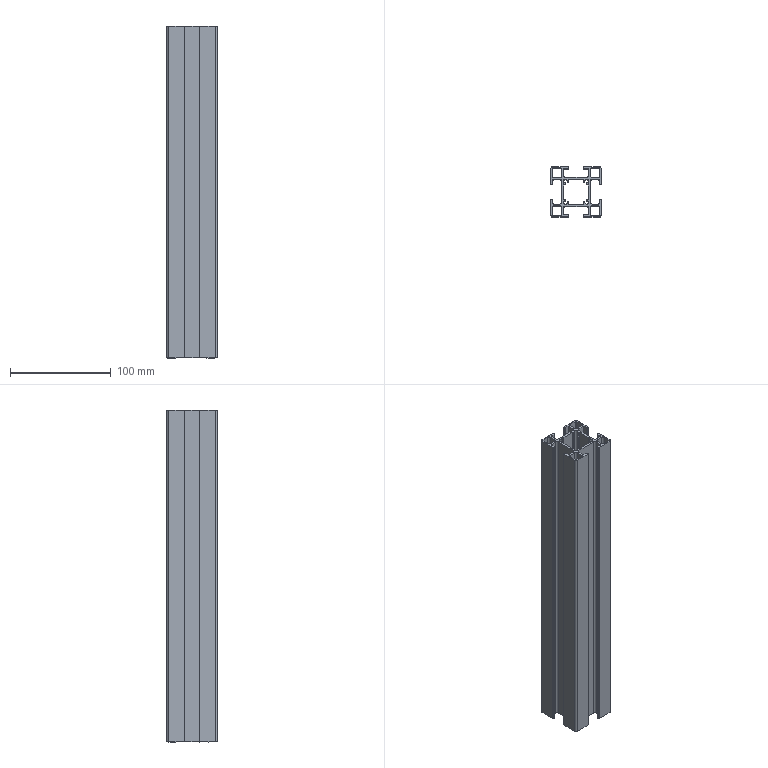Part | STEP file | 46A-00006CC11-330mm | 1 solid | 142 faces | box 50 x 50 x 330 mm | volume 193872 mm3 | cylinder 84 | plane 58 | commonest cylinder face diameters 1 x24 4 x24 1.5 x16 3.7 x8 6.7 x8 2 x4